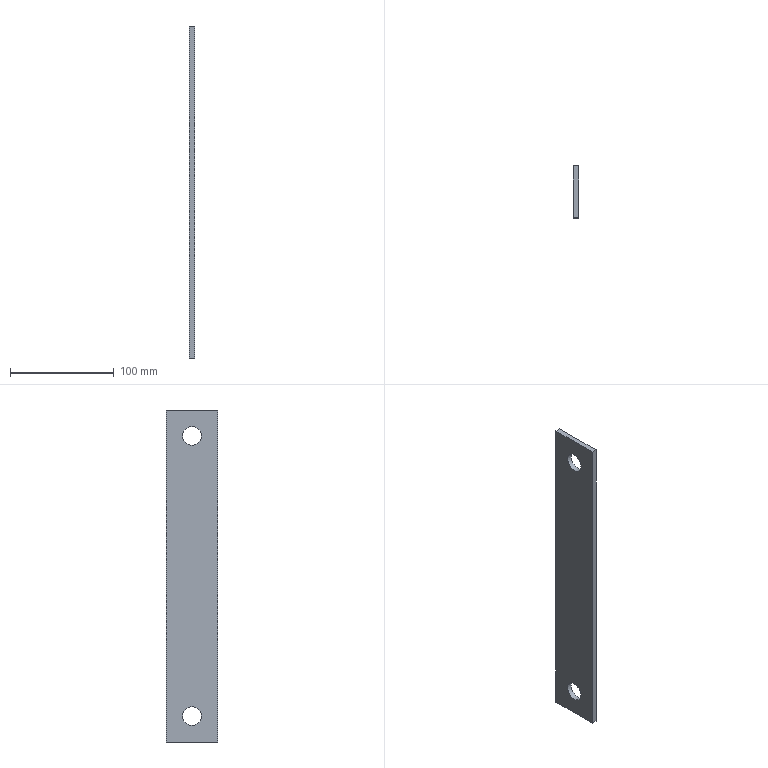Part | NX | features solid 2 | 1 solid | 8 faces | box 5 x 50 x 320 mm | volume 77455 mm3 | plane 6 | cylinder 2 | commonest cylinder face diameters 18 x2
STEP:
#1=CARTESIAN_POINT('',(505.,380.,110.));
#2=VERTEX_POINT('',#1);
#3=CARTESIAN_POINT('',(510.,380.,110.));
#4=VERTEX_POINT('',#3);
#5=CARTESIAN_POINT('',(500.,380.,110.));
#6=DIRECTION('',(-1.,0.,0.));
#7=VECTOR('',#6,1000.);
#8=LINE('',#5,#7);
#9=EDGE_CURVE('',#2,#4,#8,.F.);
#10=ORIENTED_EDGE('',*,*,#9,.T.);
#11=CARTESIAN_POINT('',(510.,430.,110.));
#12=VERTEX_POINT('',#11);
#13=CARTESIAN_POINT('',(510.,429.99,110.));
#14=DIRECTION('',(0.,-1.,0.));
#15=VECTOR('',#14,1000.);
#16=LINE('',#13,#15);
#17=EDGE_CURVE('',#12,#4,#16,.T.);
#18=ORIENTED_EDGE('',*,*,#17,.F.);
#19=CARTESIAN_POINT('',(505.,430.,110.));
#20=VERTEX_POINT('',#19);
#21=CARTESIAN_POINT('',(505.,430.,110.));
#22=DIRECTION('',(1.,0.,0.));
#23=VECTOR('',#22,1000.);
#24=LINE('',#21,#23);
#25=EDGE_CURVE('',#20,#12,#24,.T.);
#26=ORIENTED_EDGE('',*,*,#25,.F.);
#27=CARTESIAN_POINT('',(505.,429.99,110.));
#28=DIRECTION('',(0.,-1.,0.));
#29=VECTOR('',#28,1000.);
#30=LINE('',#27,#29);
#31=EDGE_CURVE('',#20,#2,#30,.T.);
#32=ORIENTED_EDGE('',*,*,#31,.T.);
#33=EDGE_LOOP('',(#10,#18,#26,#32));
#34=FACE_BOUND('',#33,.T.);
#35=CARTESIAN_POINT('',(500.,429.99,110.));
#36=DIRECTION('',(0.,0.,-1.));
#37=DIRECTION('',(0.,-1.,0.));
#38=AXIS2_PLACEMENT_3D('',#35,#36,#37);
#39=PLANE('',#38);
#40=ADVANCED_FACE('',(#34),#39,.F.);
#41=ORIENTED_EDGE('',*,*,#25,.T.);
#42=CARTESIAN_POINT('',(510.,430.,-210.));
#43=VERTEX_POINT('',#42);
#44=CARTESIAN_POINT('',(510.,430.,10.));
#45=DIRECTION('',(0.,0.,1.));
#46=VECTOR('',#45,1000.);
#47=LINE('',#44,#46);
#48=EDGE_CURVE('',#12,#43,#47,.F.);
#49=ORIENTED_EDGE('',*,*,#48,.T.);
#50=CARTESIAN_POINT('',(505.,430.,-210.));
#51=VERTEX_POINT('',#50);
#52=CARTESIAN_POINT('',(505.,430.,-210.));
#53=DIRECTION('',(-1.,0.,0.));
#54=VECTOR('',#53,1000.);
#55=LINE('',#52,#54);
#56=EDGE_CURVE('',#51,#43,#55,.F.);
#57=ORIENTED_EDGE('',*,*,#56,.F.);
#58=CARTESIAN_POINT('',(505.,430.,10.));
#59=DIRECTION('',(0.,0.,-1.));
#60=VECTOR('',#59,1000.);
#61=LINE('',#58,#60);
#62=EDGE_CURVE('',#20,#51,#61,.T.);
#63=ORIENTED_EDGE('',*,*,#62,.F.);
#64=EDGE_LOOP('',(#41,#49,#57,#63));
#65=FACE_BOUND('',#64,.T.);
#66=CARTESIAN_POINT('',(505.,430.,10.));
#67=DIRECTION('',(0.,-1.,0.));
#68=DIRECTION('',(0.,0.,-1.));
#69=AXIS2_PLACEMENT_3D('',#66,#67,#68);
#70=PLANE('',#69);
#71=ADVANCED_FACE('',(#65),#70,.F.);
#72=ORIENTED_EDGE('',*,*,#56,.T.);
#73=CARTESIAN_POINT('',(510.,380.,-210.));
#74=VERTEX_POINT('',#73);
#75=CARTESIAN_POINT('',(510.,430.,-210.));
#76=DIRECTION('',(0.,1.,0.));
#77=VECTOR('',#76,1000.);
#78=LINE('',#75,#77);
#79=EDGE_CURVE('',#43,#74,#78,.F.);
#80=ORIENTED_EDGE('',*,*,#79,.T.);
#81=CARTESIAN_POINT('',(505.,380.,-210.));
#82=VERTEX_POINT('',#81);
#83=CARTESIAN_POINT('',(505.,380.,-210.));
#84=DIRECTION('',(-1.,0.,0.));
#85=VECTOR('',#84,1000.);
#86=LINE('',#83,#85);
#87=EDGE_CURVE('',#82,#74,#86,.F.);
#88=ORIENTED_EDGE('',*,*,#87,.F.);
#89=CARTESIAN_POINT('',(505.,430.,-210.));
#90=DIRECTION('',(0.,-1.,0.));
#91=VECTOR('',#90,1000.);
#92=LINE('',#89,#91);
#93=EDGE_CURVE('',#51,#82,#92,.T.);
#94=ORIENTED_EDGE('',*,*,#93,.F.);
#95=EDGE_LOOP('',(#72,#80,#88,#94));
#96=FACE_BOUND('',#95,.T.);
#97=CARTESIAN_POINT('',(505.,430.,-210.));
#98=DIRECTION('',(0.,0.,1.));
#99=DIRECTION('',(0.,-1.,0.));
#100=AXIS2_PLACEMENT_3D('',#97,#98,#99);
#101=PLANE('',#100);
#102=ADVANCED_FACE('',(#96),#101,.F.);
#103=CARTESIAN_POINT('',(505.,380.,10.));
#104=DIRECTION('',(0.,0.,-1.));
#105=VECTOR('',#104,1000.);
#106=LINE('',#103,#105);
#107=EDGE_CURVE('',#2,#82,#106,.T.);
#108=ORIENTED_EDGE('',*,*,#107,.T.);
#109=ORIENTED_EDGE('',*,*,#87,.T.);
#110=CARTESIAN_POINT('',(510.,380.,10.));
#111=DIRECTION('',(0.,0.,1.));
#112=VECTOR('',#111,1000.);
#113=LINE('',#110,#112);
#114=EDGE_CURVE('',#4,#74,#113,.F.);
#115=ORIENTED_EDGE('',*,*,#114,.F.);
#116=ORIENTED_EDGE('',*,*,#9,.F.);
#117=EDGE_LOOP('',(#108,#109,#115,#116));
#118=FACE_BOUND('',#117,.T.);
#119=CARTESIAN_POINT('',(505.,380.,10.));
#120=DIRECTION('',(0.,-1.,0.));
#121=DIRECTION('',(0.,0.,-1.));
#122=AXIS2_PLACEMENT_3D('',#119,#120,#121);
#123=PLANE('',#122);
#124=ADVANCED_FACE('',(#118),#123,.T.);
#125=CARTESIAN_POINT('',(510.,396.,-185.));
#126=VERTEX_POINT('',#125);
#127=CARTESIAN_POINT('',(510.,405.,-185.));
#128=DIRECTION('',(-1.,0.,0.));
#129=DIRECTION('',(0.,-1.,0.));
#130=AXIS2_PLACEMENT_3D('',#127,#128,#129);
#131=CIRCLE('',#130,9.);
#132=EDGE_CURVE('',#126,#126,#131,.T.);
#133=ORIENTED_EDGE('',*,*,#132,.T.);
#134=EDGE_LOOP('',(#133));
#135=FACE_BOUND('',#134,.T.);
#136=CARTESIAN_POINT('',(510.,396.,85.));
#137=VERTEX_POINT('',#136);
#138=CARTESIAN_POINT('',(510.,405.,85.));
#139=DIRECTION('',(-1.,0.,0.));
#140=DIRECTION('',(0.,-1.,0.));
#141=AXIS2_PLACEMENT_3D('',#138,#139,#140);
#142=CIRCLE('',#141,9.);
#143=EDGE_CURVE('',#137,#137,#142,.T.);
#144=ORIENTED_EDGE('',*,*,#143,.T.);
#145=EDGE_LOOP('',(#144));
#146=FACE_BOUND('',#145,.T.);
#147=ORIENTED_EDGE('',*,*,#79,.F.);
#148=ORIENTED_EDGE('',*,*,#48,.F.);
#149=ORIENTED_EDGE('',*,*,#17,.T.);
#150=ORIENTED_EDGE('',*,*,#114,.T.);
#151=EDGE_LOOP('',(#147,#148,#149,#150));
#152=FACE_BOUND('',#151,.T.);
#153=CARTESIAN_POINT('',(510.,430.,10.));
#154=DIRECTION('',(1.,0.,0.));
#155=DIRECTION('',(0.,1.,0.));
#156=AXIS2_PLACEMENT_3D('',#153,#154,#155);
#157=PLANE('',#156);
#158=ADVANCED_FACE('',(#135,#146,#152),#157,.T.);
#159=CARTESIAN_POINT('',(505.,414.,-185.));
#160=VERTEX_POINT('',#159);
#161=CARTESIAN_POINT('',(505.,405.,-185.));
#162=DIRECTION('',(1.,0.,0.));
#163=DIRECTION('',(0.,1.,0.));
#164=AXIS2_PLACEMENT_3D('',#161,#162,#163);
#165=CIRCLE('',#164,9.);
#166=EDGE_CURVE('',#160,#160,#165,.T.);
#167=ORIENTED_EDGE('',*,*,#166,.T.);
#168=EDGE_LOOP('',(#167));
#169=FACE_BOUND('',#168,.T.);
#170=CARTESIAN_POINT('',(505.,414.,85.));
#171=VERTEX_POINT('',#170);
#172=CARTESIAN_POINT('',(505.,405.,85.));
#173=DIRECTION('',(1.,0.,0.));
#174=DIRECTION('',(0.,1.,0.));
#175=AXIS2_PLACEMENT_3D('',#172,#173,#174);
#176=CIRCLE('',#175,9.);
#177=EDGE_CURVE('',#171,#171,#176,.T.);
#178=ORIENTED_EDGE('',*,*,#177,.T.);
#179=EDGE_LOOP('',(#178));
#180=FACE_BOUND('',#179,.T.);
#181=ORIENTED_EDGE('',*,*,#93,.T.);
#182=ORIENTED_EDGE('',*,*,#107,.F.);
#183=ORIENTED_EDGE('',*,*,#31,.F.);
#184=ORIENTED_EDGE('',*,*,#62,.T.);
#185=EDGE_LOOP('',(#181,#182,#183,#184));
#186=FACE_BOUND('',#185,.T.);
#187=CARTESIAN_POINT('',(505.,430.,10.));
#188=DIRECTION('',(1.,0.,0.));
#189=DIRECTION('',(0.,1.,0.));
#190=AXIS2_PLACEMENT_3D('',#187,#188,#189);
#191=PLANE('',#190);
#192=ADVANCED_FACE('',(#169,#180,#186),#191,.F.);
#193=ORIENTED_EDGE('',*,*,#143,.F.);
#194=EDGE_LOOP('',(#193));
#195=FACE_BOUND('',#194,.T.);
#196=ORIENTED_EDGE('',*,*,#177,.F.);
#197=EDGE_LOOP('',(#196));
#198=FACE_BOUND('',#197,.T.);
#199=CARTESIAN_POINT('',(510.,405.,85.));
#200=DIRECTION('',(-1.,0.,0.));
#201=DIRECTION('',(0.,-1.,0.));
#202=AXIS2_PLACEMENT_3D('',#199,#200,#201);
#203=CYLINDRICAL_SURFACE('',#202,9.);
#204=ADVANCED_FACE('',(#195,#198),#203,.F.);
#205=ORIENTED_EDGE('',*,*,#132,.F.);
#206=EDGE_LOOP('',(#205));
#207=FACE_BOUND('',#206,.T.);
#208=ORIENTED_EDGE('',*,*,#166,.F.);
#209=EDGE_LOOP('',(#208));
#210=FACE_BOUND('',#209,.T.);
#211=CARTESIAN_POINT('',(510.,405.,-185.));
#212=DIRECTION('',(-1.,0.,0.));
#213=DIRECTION('',(0.,-1.,0.));
#214=AXIS2_PLACEMENT_3D('',#211,#212,#213);
#215=CYLINDRICAL_SURFACE('',#214,9.);
#216=ADVANCED_FACE('',(#207,#210),#215,.F.);
#217=CLOSED_SHELL('',(#40,#71,#102,#124,#158,#192,#204,#216));
#218=MANIFOLD_SOLID_BREP('',#217);
#219=(LENGTH_UNIT()NAMED_UNIT(*)SI_UNIT(.MILLI.,.METRE.));
#220=UNCERTAINTY_MEASURE_WITH_UNIT(LENGTH_MEASURE(0.00001),#219,'','');
#221=(NAMED_UNIT(*)PLANE_ANGLE_UNIT()SI_UNIT($,.RADIAN.));
#222=(NAMED_UNIT(*)SI_UNIT($,.STERADIAN.)SOLID_ANGLE_UNIT());
#223=(GEOMETRIC_REPRESENTATION_CONTEXT(3)GLOBAL_UNCERTAINTY_ASSIGNED_CONTEXT((#220))GLOBAL_UNIT_ASSIGNED_CONTEXT((#219,#221,#222))REPRESENTATION_CONTEXT('',''));
#224=ADVANCED_BREP_SHAPE_REPRESENTATION('',(#218),#223);